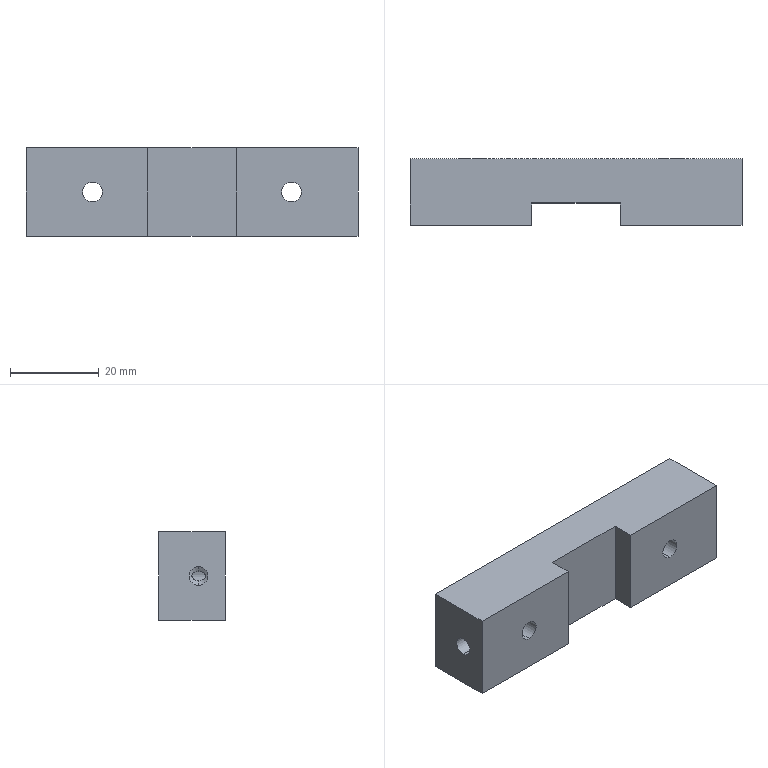Part | STEP file | push seat | 1 solid | 24 faces | box 75 x 15 x 20 mm | volume 19572 mm3 | plane 12 | cylinder 10 | cone 2 | commonest cylinder face diameters 4.5 x4 8 x4 4.2 x2